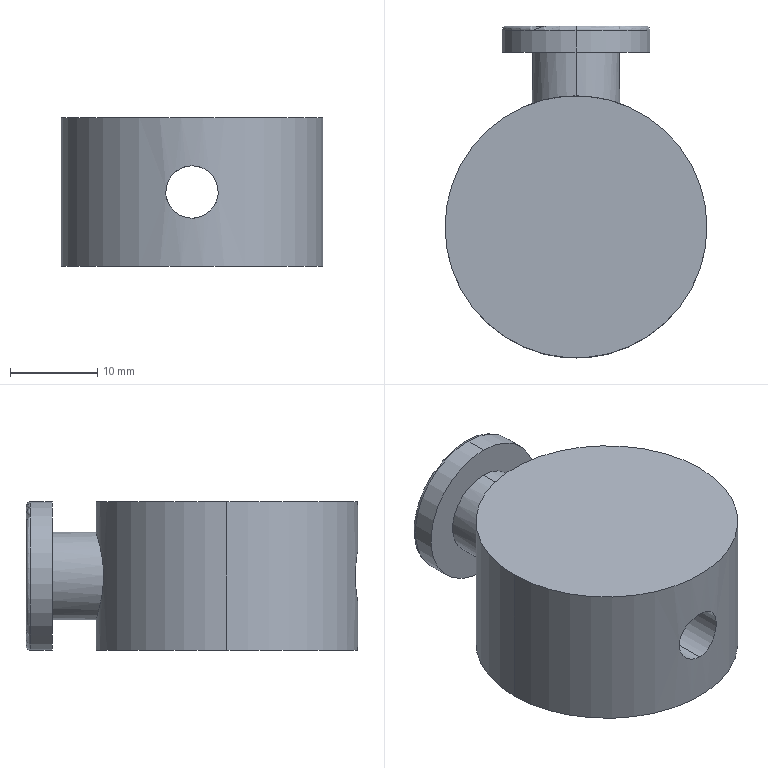Part | SolidWorks | features ICE 3, Extrusion 1, Fillet 1 | 1 solid | 14 faces | box 30 x 38 x 17 mm | volume 12032 mm3 | cylinder 8 | plane 4 | torus 2 | commonest cylinder face diameters 6 x2 10 x2 17 x2 30 x2
STEP:
#1=CARTESIAN_POINT('',(0.,22.5,-8.5));
#2=VERTEX_POINT('',#1);
#3=CARTESIAN_POINT('',(0.,22.5,8.5));
#4=VERTEX_POINT('',#3);
#5=CARTESIAN_POINT('',(0.,22.5,0.));
#6=DIRECTION('',(0.,-1.,0.));
#7=DIRECTION('',(0.,0.,1.));
#8=AXIS2_PLACEMENT_3D('',#5,#6,#7);
#9=CIRCLE('',#8,8.5);
#10=EDGE_CURVE('',#2,#4,#9,.T.);
#11=ORIENTED_EDGE('',*,*,#10,.F.);
#12=CARTESIAN_POINT('',(0.,23.,-8.));
#13=VERTEX_POINT('',#12);
#14=CARTESIAN_POINT('',(0.,22.5,-8.));
#15=DIRECTION('',(1.,0.,0.));
#16=DIRECTION('',(0.,0.,-1.));
#17=AXIS2_PLACEMENT_3D('',#14,#15,#16);
#18=CIRCLE('',#17,0.5);
#19=EDGE_CURVE('',#2,#13,#18,.T.);
#20=ORIENTED_EDGE('',*,*,#19,.T.);
#21=CARTESIAN_POINT('',(0.,23.,8.));
#22=VERTEX_POINT('',#21);
#23=CARTESIAN_POINT('',(0.,23.,0.));
#24=DIRECTION('',(0.,1.,0.));
#25=DIRECTION('',(0.,0.,1.));
#26=AXIS2_PLACEMENT_3D('',#23,#24,#25);
#27=CIRCLE('',#26,8.);
#28=EDGE_CURVE('',#22,#13,#27,.T.);
#29=ORIENTED_EDGE('',*,*,#28,.F.);
#30=CARTESIAN_POINT('',(0.,22.5,8.));
#31=DIRECTION('',(-1.,0.,0.));
#32=DIRECTION('',(0.,0.,1.));
#33=AXIS2_PLACEMENT_3D('',#30,#31,#32);
#34=CIRCLE('',#33,0.5);
#35=EDGE_CURVE('',#4,#22,#34,.T.);
#36=ORIENTED_EDGE('',*,*,#35,.F.);
#37=EDGE_LOOP('',(#11,#20,#29,#36));
#38=FACE_OUTER_BOUND('',#37,.T.);
#39=CARTESIAN_POINT('',(0.,22.5,0.));
#40=DIRECTION('',(0.,1.,0.));
#41=DIRECTION('',(0.,0.,1.));
#42=AXIS2_PLACEMENT_3D('',#39,#40,#41);
#43=TOROIDAL_SURFACE('',#42,8.,0.5);
#44=ADVANCED_FACE('',(#38),#43,.T.);
#45=ORIENTED_EDGE('',*,*,#10,.T.);
#46=CARTESIAN_POINT('',(0.,20.,8.5));
#47=VERTEX_POINT('',#46);
#48=CARTESIAN_POINT('',(0.,23.,8.5));
#49=DIRECTION('',(0.,-1.,0.));
#50=VECTOR('',#49,1000.);
#51=LINE('',#48,#50);
#52=EDGE_CURVE('',#4,#47,#51,.T.);
#53=ORIENTED_EDGE('',*,*,#52,.T.);
#54=CARTESIAN_POINT('',(0.,20.,-8.5));
#55=VERTEX_POINT('',#54);
#56=CARTESIAN_POINT('',(0.,20.,0.));
#57=DIRECTION('',(0.,1.,0.));
#58=DIRECTION('',(0.,0.,1.));
#59=AXIS2_PLACEMENT_3D('',#56,#57,#58);
#60=CIRCLE('',#59,8.5);
#61=EDGE_CURVE('',#47,#55,#60,.T.);
#62=ORIENTED_EDGE('',*,*,#61,.T.);
#63=CARTESIAN_POINT('',(0.,23.,-8.5));
#64=DIRECTION('',(0.,-1.,0.));
#65=VECTOR('',#64,1000.);
#66=LINE('',#63,#65);
#67=EDGE_CURVE('',#2,#55,#66,.T.);
#68=ORIENTED_EDGE('',*,*,#67,.F.);
#69=EDGE_LOOP('',(#45,#53,#62,#68));
#70=FACE_OUTER_BOUND('',#69,.T.);
#71=CARTESIAN_POINT('',(0.,23.,0.));
#72=DIRECTION('',(0.,-1.,0.));
#73=DIRECTION('',(0.,0.,-1.));
#74=AXIS2_PLACEMENT_3D('',#71,#72,#73);
#75=CYLINDRICAL_SURFACE('',#74,8.5);
#76=ADVANCED_FACE('',(#70),#75,.T.);
#77=CARTESIAN_POINT('',(0.,15.,5.));
#78=VERTEX_POINT('',#77);
#79=CARTESIAN_POINT('',(0.,15.,-5.));
#80=VERTEX_POINT('',#79);
#81=CARTESIAN_POINT('',(0.,15.,5.));
#82=CARTESIAN_POINT('',(0.3329,15.,5.));
#83=CARTESIAN_POINT('',(0.6598,14.989,4.967));
#84=CARTESIAN_POINT('',(1.302,14.947,4.839));
#85=CARTESIAN_POINT('',(1.621,14.915,4.741));
#86=CARTESIAN_POINT('',(2.226,14.837,4.489));
#87=CARTESIAN_POINT('',(2.512,14.791,4.335));
#88=CARTESIAN_POINT('',(3.054,14.688,3.972));
#89=CARTESIAN_POINT('',(3.308,14.633,3.763));
#90=CARTESIAN_POINT('',(3.766,14.521,3.305));
#91=CARTESIAN_POINT('',(3.972,14.466,3.055));
#92=CARTESIAN_POINT('',(4.337,14.36,2.509));
#93=CARTESIAN_POINT('',(4.491,14.313,2.222));
#94=CARTESIAN_POINT('',(4.678,14.252,1.772));
#95=CARTESIAN_POINT('',(4.734,14.234,1.618));
#96=CARTESIAN_POINT('',(4.83,14.201,1.304));
#97=CARTESIAN_POINT('',(4.871,14.187,1.142));
#98=CARTESIAN_POINT('',(4.968,14.154,0.6573));
#99=CARTESIAN_POINT('',(5.,14.142,0.3313));
#100=CARTESIAN_POINT('',(5.,14.142,-0.3263));
#101=CARTESIAN_POINT('',(4.967,14.154,-0.6604));
#102=CARTESIAN_POINT('',(4.838,14.198,-1.304));
#103=CARTESIAN_POINT('',(4.743,14.231,-1.617));
#104=CARTESIAN_POINT('',(4.49,14.313,-2.225));
#105=CARTESIAN_POINT('',(4.335,14.361,-2.513));
#106=CARTESIAN_POINT('',(3.973,14.465,-3.052));
#107=CARTESIAN_POINT('',(3.764,14.522,-3.307));
#108=CARTESIAN_POINT('',(3.304,14.634,-3.767));
#109=CARTESIAN_POINT('',(3.054,14.688,-3.972));
#110=CARTESIAN_POINT('',(2.514,14.79,-4.334));
#111=CARTESIAN_POINT('',(2.221,14.838,-4.491));
#112=CARTESIAN_POINT('',(1.619,14.915,-4.742));
#113=CARTESIAN_POINT('',(1.307,14.946,-4.837));
#114=CARTESIAN_POINT('',(0.8213,14.978,-4.935));
#115=CARTESIAN_POINT('',(0.6562,14.987,-4.959));
#116=CARTESIAN_POINT('',(0.328,14.997,-4.992));
#117=CARTESIAN_POINT('',(0.164,15.,-5.));
#118=CARTESIAN_POINT('',(0.,15.,-5.));
#119=B_SPLINE_CURVE_WITH_KNOTS('',3,(#81,#82,#83,#84,#85,#86,#87,#88,#89,#90,#91,#92,#93,#94,#95,#96,#97,#98,#99,#100,#101,#102,#103,#104,#105,#106,#107,#108,#109,#110,#111,#112,#113,#114,#115,#116,#117,#118),.UNSPECIFIED.,.F.,.F.,(4,2,2,2,2,2,2,2,2,2,2,2,2,2,2,2,2,2,4),(0.,0.0009841,0.001968,0.002952,0.003936,0.004921,0.005905,0.006397,0.006889,0.007873,0.008857,0.009841,0.01083,0.01181,0.01279,0.01378,0.01476,0.01525,0.01575),.UNSPECIFIED.);
#120=EDGE_CURVE('',#78,#80,#119,.T.);
#121=ORIENTED_EDGE('',*,*,#120,.T.);
#122=CARTESIAN_POINT('',(0.,20.,-5.));
#123=VERTEX_POINT('',#122);
#124=CARTESIAN_POINT('',(0.,-15.001,-5.));
#125=DIRECTION('',(0.,1.,0.));
#126=VECTOR('',#125,1000.);
#127=LINE('',#124,#126);
#128=EDGE_CURVE('',#80,#123,#127,.T.);
#129=ORIENTED_EDGE('',*,*,#128,.T.);
#130=CARTESIAN_POINT('',(0.,20.,5.));
#131=VERTEX_POINT('',#130);
#132=CARTESIAN_POINT('',(0.,20.,0.));
#133=DIRECTION('',(0.,1.,0.));
#134=DIRECTION('',(0.,0.,1.));
#135=AXIS2_PLACEMENT_3D('',#132,#133,#134);
#136=CIRCLE('',#135,5.);
#137=EDGE_CURVE('',#131,#123,#136,.T.);
#138=ORIENTED_EDGE('',*,*,#137,.F.);
#139=CARTESIAN_POINT('',(0.,-15.001,5.));
#140=DIRECTION('',(0.,1.,0.));
#141=VECTOR('',#140,1000.);
#142=LINE('',#139,#141);
#143=EDGE_CURVE('',#78,#131,#142,.T.);
#144=ORIENTED_EDGE('',*,*,#143,.F.);
#145=EDGE_LOOP('',(#121,#129,#138,#144));
#146=FACE_OUTER_BOUND('',#145,.T.);
#147=CARTESIAN_POINT('',(0.,-15.001,0.));
#148=DIRECTION('',(0.,1.,0.));
#149=DIRECTION('',(0.,0.,1.));
#150=AXIS2_PLACEMENT_3D('',#147,#148,#149);
#151=CYLINDRICAL_SURFACE('',#150,5.);
#152=ADVANCED_FACE('',(#146),#151,.T.);
#153=CARTESIAN_POINT('',(0.,-15.,-3.));
#154=VERTEX_POINT('',#153);
#155=CARTESIAN_POINT('',(0.,-15.,3.));
#156=VERTEX_POINT('',#155);
#157=CARTESIAN_POINT('',(0.,-15.,-3.));
#158=CARTESIAN_POINT('',(-0.196,-15.,-3.));
#159=CARTESIAN_POINT('',(-0.3912,-14.996,-2.981));
#160=CARTESIAN_POINT('',(-0.7798,-14.981,-2.904));
#161=CARTESIAN_POINT('',(-0.9683,-14.97,-2.846));
#162=CARTESIAN_POINT('',(-1.329,-14.942,-2.696));
#163=CARTESIAN_POINT('',(-1.505,-14.925,-2.603));
#164=CARTESIAN_POINT('',(-1.831,-14.889,-2.384));
#165=CARTESIAN_POINT('',(-1.982,-14.869,-2.261));
#166=CARTESIAN_POINT('',(-2.258,-14.83,-1.984));
#167=CARTESIAN_POINT('',(-2.385,-14.81,-1.83));
#168=CARTESIAN_POINT('',(-2.602,-14.773,-1.506));
#169=CARTESIAN_POINT('',(-2.694,-14.756,-1.334));
#170=CARTESIAN_POINT('',(-2.846,-14.728,-0.9697));
#171=CARTESIAN_POINT('',(-2.903,-14.716,-0.78));
#172=CARTESIAN_POINT('',(-2.98,-14.701,-0.3963));
#173=CARTESIAN_POINT('',(-3.,-14.697,-0.1996));
#174=CARTESIAN_POINT('',(-3.,-14.697,0.1966));
#175=CARTESIAN_POINT('',(-2.981,-14.701,0.3917));
#176=CARTESIAN_POINT('',(-2.904,-14.716,0.7761));
#177=CARTESIAN_POINT('',(-2.847,-14.728,0.9674));
#178=CARTESIAN_POINT('',(-2.696,-14.756,1.33));
#179=CARTESIAN_POINT('',(-2.604,-14.773,1.502));
#180=CARTESIAN_POINT('',(-2.386,-14.809,1.829));
#181=CARTESIAN_POINT('',(-2.26,-14.829,1.982));
#182=CARTESIAN_POINT('',(-1.847,-14.888,2.396));
#183=CARTESIAN_POINT('',(-1.513,-14.928,2.62));
#184=CARTESIAN_POINT('',(-0.9723,-14.97,2.845));
#185=CARTESIAN_POINT('',(-0.782,-14.981,2.903));
#186=CARTESIAN_POINT('',(-0.3948,-14.996,2.98));
#187=CARTESIAN_POINT('',(-0.1987,-15.,3.));
#188=CARTESIAN_POINT('',(0.,-15.,3.));
#189=B_SPLINE_CURVE_WITH_KNOTS('',3,(#157,#158,#159,#160,#161,#162,#163,#164,#165,#166,#167,#168,#169,#170,#171,#172,#173,#174,#175,#176,#177,#178,#179,#180,#181,#182,#183,#184,#185,#186,#187,#188),.UNSPECIFIED.,.F.,.F.,(4,2,2,2,2,2,2,2,2,2,2,2,2,2,2,4),(0.009403,0.009991,0.01058,0.01117,0.01175,0.01234,0.01293,0.01352,0.0141,0.01469,0.01528,0.01587,0.01645,0.01763,0.01822,0.0188),.UNSPECIFIED.);
#190=EDGE_CURVE('',#154,#156,#189,.T.);
#191=ORIENTED_EDGE('',*,*,#190,.F.);
#192=CARTESIAN_POINT('',(0.,23.,-3.));
#193=VERTEX_POINT('',#192);
#194=CARTESIAN_POINT('',(0.,-15.,-3.));
#195=DIRECTION('',(0.,1.,0.));
#196=VECTOR('',#195,1000.);
#197=LINE('',#194,#196);
#198=EDGE_CURVE('',#154,#193,#197,.T.);
#199=ORIENTED_EDGE('',*,*,#198,.T.);
#200=CARTESIAN_POINT('',(0.,23.,3.));
#201=VERTEX_POINT('',#200);
#202=CARTESIAN_POINT('',(0.,23.,0.));
#203=DIRECTION('',(0.,1.,0.));
#204=DIRECTION('',(0.,0.,1.));
#205=AXIS2_PLACEMENT_3D('',#202,#203,#204);
#206=CIRCLE('',#205,3.);
#207=EDGE_CURVE('',#193,#201,#206,.T.);
#208=ORIENTED_EDGE('',*,*,#207,.T.);
#209=CARTESIAN_POINT('',(0.,-15.,3.));
#210=DIRECTION('',(0.,1.,0.));
#211=VECTOR('',#210,1000.);
#212=LINE('',#209,#211);
#213=EDGE_CURVE('',#156,#201,#212,.T.);
#214=ORIENTED_EDGE('',*,*,#213,.F.);
#215=EDGE_LOOP('',(#191,#199,#208,#214));
#216=FACE_OUTER_BOUND('',#215,.T.);
#217=CARTESIAN_POINT('',(0.,-15.,0.));
#218=DIRECTION('',(0.,1.,0.));
#219=DIRECTION('',(0.,0.,1.));
#220=AXIS2_PLACEMENT_3D('',#217,#218,#219);
#221=CYLINDRICAL_SURFACE('',#220,3.);
#222=ADVANCED_FACE('',(#216),#221,.F.);
#223=ORIENTED_EDGE('',*,*,#120,.F.);
#224=CARTESIAN_POINT('',(0.,15.,-5.));
#225=CARTESIAN_POINT('',(-0.3279,15.,-5.));
#226=CARTESIAN_POINT('',(-0.6581,14.989,-4.968));
#227=CARTESIAN_POINT('',(-1.307,14.947,-4.838));
#228=CARTESIAN_POINT('',(-1.619,14.915,-4.742));
#229=CARTESIAN_POINT('',(-2.223,14.838,-4.491));
#230=CARTESIAN_POINT('',(-2.515,14.79,-4.334));
#231=CARTESIAN_POINT('',(-3.055,14.688,-3.971));
#232=CARTESIAN_POINT('',(-3.305,14.633,-3.766));
#233=CARTESIAN_POINT('',(-3.767,14.521,-3.304));
#234=CARTESIAN_POINT('',(-3.974,14.465,-3.051));
#235=CARTESIAN_POINT('',(-4.335,14.361,-2.513));
#236=CARTESIAN_POINT('',(-4.49,14.313,-2.224));
#237=CARTESIAN_POINT('',(-4.743,14.231,-1.616));
#238=CARTESIAN_POINT('',(-4.838,14.199,-1.304));
#239=CARTESIAN_POINT('',(-4.967,14.154,-0.6625));
#240=CARTESIAN_POINT('',(-5.,14.142,-0.3289));
#241=CARTESIAN_POINT('',(-5.,14.142,0.3301));
#242=CARTESIAN_POINT('',(-4.968,14.154,0.6563));
#243=CARTESIAN_POINT('',(-4.871,14.187,1.141));
#244=CARTESIAN_POINT('',(-4.83,14.201,1.302));
#245=CARTESIAN_POINT('',(-4.734,14.233,1.617));
#246=CARTESIAN_POINT('',(-4.679,14.252,1.771));
#247=CARTESIAN_POINT('',(-4.491,14.313,2.223));
#248=CARTESIAN_POINT('',(-4.336,14.361,2.512));
#249=CARTESIAN_POINT('',(-3.971,14.466,3.056));
#250=CARTESIAN_POINT('',(-3.765,14.522,3.306));
#251=CARTESIAN_POINT('',(-3.307,14.633,3.764));
#252=CARTESIAN_POINT('',(-3.052,14.689,3.974));
#253=CARTESIAN_POINT('',(-2.511,14.791,4.336));
#254=CARTESIAN_POINT('',(-2.225,14.837,4.489));
#255=CARTESIAN_POINT('',(-1.772,14.896,4.678));
#256=CARTESIAN_POINT('',(-1.616,14.914,4.735));
#257=CARTESIAN_POINT('',(-1.301,14.944,4.831));
#258=CARTESIAN_POINT('',(-1.142,14.957,4.871));
#259=CARTESIAN_POINT('',(-0.6599,14.989,4.967));
#260=CARTESIAN_POINT('',(-0.3328,15.,5.));
#261=CARTESIAN_POINT('',(0.,15.,5.));
#262=B_SPLINE_CURVE_WITH_KNOTS('',3,(#224,#225,#226,#227,#228,#229,#230,#231,#232,#233,#234,#235,#236,#237,#238,#239,#240,#241,#242,#243,#244,#245,#246,#247,#248,#249,#250,#251,#252,#253,#254,#255,#256,#257,#258,#259,#260,#261),.UNSPECIFIED.,.F.,.F.,(4,2,2,2,2,2,2,2,2,2,2,2,2,2,2,2,2,2,4),(0.01575,0.01673,0.01771,0.0187,0.01968,0.02067,0.02165,0.02263,0.02362,0.0246,0.02509,0.02558,0.02657,0.02755,0.02854,0.02952,0.03001,0.0305,0.03149),.UNSPECIFIED.);
#263=EDGE_CURVE('',#80,#78,#262,.T.);
#264=ORIENTED_EDGE('',*,*,#263,.F.);
#265=EDGE_LOOP('',(#223,#264));
#266=FACE_BOUND('',#265,.T.);
#267=CARTESIAN_POINT('',(15.,0.,8.5));
#268=VERTEX_POINT('',#267);
#269=CARTESIAN_POINT('',(-15.,0.,8.5));
#270=VERTEX_POINT('',#269);
#271=CARTESIAN_POINT('',(0.,0.,8.5));
#272=DIRECTION('',(0.,0.,1.));
#273=DIRECTION('',(1.,0.,0.));
#274=AXIS2_PLACEMENT_3D('',#271,#272,#273);
#275=CIRCLE('',#274,15.);
#276=EDGE_CURVE('',#268,#270,#275,.T.);
#277=ORIENTED_EDGE('',*,*,#276,.F.);
#278=CARTESIAN_POINT('',(15.,0.,-8.5));
#279=VERTEX_POINT('',#278);
#280=CARTESIAN_POINT('',(15.,0.,8.5));
#281=DIRECTION('',(0.,0.,-1.));
#282=VECTOR('',#281,1000.);
#283=LINE('',#280,#282);
#284=EDGE_CURVE('',#268,#279,#283,.T.);
#285=ORIENTED_EDGE('',*,*,#284,.T.);
#286=CARTESIAN_POINT('',(-15.,0.,-8.5));
#287=VERTEX_POINT('',#286);
#288=CARTESIAN_POINT('',(0.,0.,-8.5));
#289=DIRECTION('',(0.,0.,1.));
#290=DIRECTION('',(1.,0.,0.));
#291=AXIS2_PLACEMENT_3D('',#288,#289,#290);
#292=CIRCLE('',#291,15.);
#293=EDGE_CURVE('',#279,#287,#292,.T.);
#294=ORIENTED_EDGE('',*,*,#293,.T.);
#295=CARTESIAN_POINT('',(-15.,0.,8.5));
#296=DIRECTION('',(0.,0.,-1.));
#297=VECTOR('',#296,1000.);
#298=LINE('',#295,#297);
#299=EDGE_CURVE('',#270,#287,#298,.T.);
#300=ORIENTED_EDGE('',*,*,#299,.F.);
#301=EDGE_LOOP('',(#277,#285,#294,#300));
#302=FACE_OUTER_BOUND('',#301,.T.);
#303=CARTESIAN_POINT('',(0.,0.,8.5));
#304=DIRECTION('',(0.,0.,-1.));
#305=DIRECTION('',(-1.,0.,0.));
#306=AXIS2_PLACEMENT_3D('',#303,#304,#305);
#307=CYLINDRICAL_SURFACE('',#306,15.);
#308=ADVANCED_FACE('',(#266,#302),#307,.T.);
#309=ORIENTED_EDGE('',*,*,#284,.F.);
#310=CARTESIAN_POINT('',(0.,0.,8.5));
#311=DIRECTION('',(0.,0.,1.));
#312=DIRECTION('',(1.,0.,0.));
#313=AXIS2_PLACEMENT_3D('',#310,#311,#312);
#314=CIRCLE('',#313,15.);
#315=EDGE_CURVE('',#270,#268,#314,.T.);
#316=ORIENTED_EDGE('',*,*,#315,.F.);
#317=ORIENTED_EDGE('',*,*,#299,.T.);
#318=CARTESIAN_POINT('',(0.,0.,-8.5));
#319=DIRECTION('',(0.,0.,1.));
#320=DIRECTION('',(1.,0.,0.));
#321=AXIS2_PLACEMENT_3D('',#318,#319,#320);
#322=CIRCLE('',#321,15.);
#323=EDGE_CURVE('',#287,#279,#322,.T.);
#324=ORIENTED_EDGE('',*,*,#323,.T.);
#325=EDGE_LOOP('',(#309,#316,#317,#324));
#326=FACE_OUTER_BOUND('',#325,.T.);
#327=CARTESIAN_POINT('',(0.,-15.,3.));
#328=CARTESIAN_POINT('',(0.1988,-15.,3.));
#329=CARTESIAN_POINT('',(0.3941,-14.996,2.98));
#330=CARTESIAN_POINT('',(0.7782,-14.981,2.904));
#331=CARTESIAN_POINT('',(0.9691,-14.97,2.846));
#332=CARTESIAN_POINT('',(1.332,-14.942,2.695));
#333=CARTESIAN_POINT('',(1.504,-14.925,2.603));
#334=CARTESIAN_POINT('',(1.83,-14.889,2.385));
#335=CARTESIAN_POINT('',(1.984,-14.869,2.259));
#336=CARTESIAN_POINT('',(2.26,-14.829,1.983));
#337=CARTESIAN_POINT('',(2.384,-14.81,1.832));
#338=CARTESIAN_POINT('',(2.603,-14.773,1.504));
#339=CARTESIAN_POINT('',(2.696,-14.756,1.33));
#340=CARTESIAN_POINT('',(2.846,-14.728,0.9696));
#341=CARTESIAN_POINT('',(2.904,-14.716,0.7799));
#342=CARTESIAN_POINT('',(2.981,-14.701,0.3924));
#343=CARTESIAN_POINT('',(3.,-14.697,0.1974));
#344=CARTESIAN_POINT('',(3.,-14.697,-0.195));
#345=CARTESIAN_POINT('',(2.98,-14.701,-0.3944));
#346=CARTESIAN_POINT('',(2.904,-14.716,-0.7796));
#347=CARTESIAN_POINT('',(2.847,-14.728,-0.9668));
#348=CARTESIAN_POINT('',(2.696,-14.756,-1.331));
#349=CARTESIAN_POINT('',(2.602,-14.773,-1.506));
#350=CARTESIAN_POINT('',(2.385,-14.81,-1.83));
#351=CARTESIAN_POINT('',(2.261,-14.829,-1.982));
#352=CARTESIAN_POINT('',(1.982,-14.869,-2.261));
#353=CARTESIAN_POINT('',(1.831,-14.889,-2.385));
#354=CARTESIAN_POINT('',(1.506,-14.925,-2.602));
#355=CARTESIAN_POINT('',(1.331,-14.942,-2.696));
#356=CARTESIAN_POINT('',(0.9679,-14.97,-2.846));
#357=CARTESIAN_POINT('',(0.7808,-14.981,-2.903));
#358=CARTESIAN_POINT('',(0.3952,-14.996,-2.98));
#359=CARTESIAN_POINT('',(0.1961,-15.,-3.));
#360=CARTESIAN_POINT('',(0.,-15.,-3.));
#361=B_SPLINE_CURVE_WITH_KNOTS('',3,(#327,#328,#329,#330,#331,#332,#333,#334,#335,#336,#337,#338,#339,#340,#341,#342,#343,#344,#345,#346,#347,#348,#349,#350,#351,#352,#353,#354,#355,#356,#357,#358,#359,#360),.UNSPECIFIED.,.F.,.F.,(4,2,2,2,2,2,2,2,2,2,2,2,2,2,2,2,4),(0.,0.0005877,0.001175,0.001763,0.002351,0.002938,0.003526,0.004114,0.004702,0.005289,0.005877,0.006465,0.007052,0.00764,0.008228,0.008815,0.009403),.UNSPECIFIED.);
#362=EDGE_CURVE('',#156,#154,#361,.T.);
#363=ORIENTED_EDGE('',*,*,#362,.T.);
#364=ORIENTED_EDGE('',*,*,#190,.T.);
#365=EDGE_LOOP('',(#363,#364));
#366=FACE_BOUND('',#365,.T.);
#367=CARTESIAN_POINT('',(0.,0.,8.5));
#368=DIRECTION('',(0.,0.,-1.));
#369=DIRECTION('',(-1.,0.,0.));
#370=AXIS2_PLACEMENT_3D('',#367,#368,#369);
#371=CYLINDRICAL_SURFACE('',#370,15.);
#372=ADVANCED_FACE('',(#326,#366),#371,.T.);
#373=ORIENTED_EDGE('',*,*,#315,.T.);
#374=ORIENTED_EDGE('',*,*,#276,.T.);
#375=EDGE_LOOP('',(#373,#374));
#376=FACE_OUTER_BOUND('',#375,.T.);
#377=CARTESIAN_POINT('',(0.,0.,8.5));
#378=DIRECTION('',(0.,0.,1.));
#379=DIRECTION('',(1.,0.,0.));
#380=AXIS2_PLACEMENT_3D('',#377,#378,#379);
#381=PLANE('',#380);
#382=ADVANCED_FACE('',(#376),#381,.T.);
#383=ORIENTED_EDGE('',*,*,#323,.F.);
#384=ORIENTED_EDGE('',*,*,#293,.F.);
#385=EDGE_LOOP('',(#383,#384));
#386=FACE_OUTER_BOUND('',#385,.T.);
#387=CARTESIAN_POINT('',(0.,0.,-8.5));
#388=DIRECTION('',(0.,0.,1.));
#389=DIRECTION('',(1.,0.,0.));
#390=AXIS2_PLACEMENT_3D('',#387,#388,#389);
#391=PLANE('',#390);
#392=ADVANCED_FACE('',(#386),#391,.F.);
#393=ORIENTED_EDGE('',*,*,#198,.F.);
#394=ORIENTED_EDGE('',*,*,#362,.F.);
#395=ORIENTED_EDGE('',*,*,#213,.T.);
#396=CARTESIAN_POINT('',(0.,23.,0.));
#397=DIRECTION('',(0.,1.,0.));
#398=DIRECTION('',(0.,0.,1.));
#399=AXIS2_PLACEMENT_3D('',#396,#397,#398);
#400=CIRCLE('',#399,3.);
#401=EDGE_CURVE('',#201,#193,#400,.T.);
#402=ORIENTED_EDGE('',*,*,#401,.T.);
#403=EDGE_LOOP('',(#393,#394,#395,#402));
#404=FACE_OUTER_BOUND('',#403,.T.);
#405=CARTESIAN_POINT('',(0.,-15.,0.));
#406=DIRECTION('',(0.,1.,0.));
#407=DIRECTION('',(0.,0.,1.));
#408=AXIS2_PLACEMENT_3D('',#405,#406,#407);
#409=CYLINDRICAL_SURFACE('',#408,3.);
#410=ADVANCED_FACE('',(#404),#409,.F.);
#411=ORIENTED_EDGE('',*,*,#128,.F.);
#412=ORIENTED_EDGE('',*,*,#263,.T.);
#413=ORIENTED_EDGE('',*,*,#143,.T.);
#414=CARTESIAN_POINT('',(0.,20.,0.));
#415=DIRECTION('',(0.,1.,0.));
#416=DIRECTION('',(0.,0.,1.));
#417=AXIS2_PLACEMENT_3D('',#414,#415,#416);
#418=CIRCLE('',#417,5.);
#419=EDGE_CURVE('',#123,#131,#418,.T.);
#420=ORIENTED_EDGE('',*,*,#419,.F.);
#421=EDGE_LOOP('',(#411,#412,#413,#420));
#422=FACE_OUTER_BOUND('',#421,.T.);
#423=CARTESIAN_POINT('',(0.,-15.001,0.));
#424=DIRECTION('',(0.,1.,0.));
#425=DIRECTION('',(0.,0.,1.));
#426=AXIS2_PLACEMENT_3D('',#423,#424,#425);
#427=CYLINDRICAL_SURFACE('',#426,5.);
#428=ADVANCED_FACE('',(#422),#427,.T.);
#429=ORIENTED_EDGE('',*,*,#28,.T.);
#430=CARTESIAN_POINT('',(0.,23.,0.));
#431=DIRECTION('',(0.,1.,0.));
#432=DIRECTION('',(0.,0.,1.));
#433=AXIS2_PLACEMENT_3D('',#430,#431,#432);
#434=CIRCLE('',#433,8.);
#435=EDGE_CURVE('',#13,#22,#434,.T.);
#436=ORIENTED_EDGE('',*,*,#435,.T.);
#437=EDGE_LOOP('',(#429,#436));
#438=FACE_OUTER_BOUND('',#437,.T.);
#439=ORIENTED_EDGE('',*,*,#401,.F.);
#440=ORIENTED_EDGE('',*,*,#207,.F.);
#441=EDGE_LOOP('',(#439,#440));
#442=FACE_BOUND('',#441,.T.);
#443=CARTESIAN_POINT('',(0.,23.,0.));
#444=DIRECTION('',(0.,1.,0.));
#445=DIRECTION('',(0.,0.,1.));
#446=AXIS2_PLACEMENT_3D('',#443,#444,#445);
#447=PLANE('',#446);
#448=ADVANCED_FACE('',(#438,#442),#447,.T.);
#449=ORIENTED_EDGE('',*,*,#137,.T.);
#450=ORIENTED_EDGE('',*,*,#419,.T.);
#451=EDGE_LOOP('',(#449,#450));
#452=FACE_BOUND('',#451,.T.);
#453=CARTESIAN_POINT('',(0.,20.,0.));
#454=DIRECTION('',(0.,1.,0.));
#455=DIRECTION('',(0.,0.,1.));
#456=AXIS2_PLACEMENT_3D('',#453,#454,#455);
#457=CIRCLE('',#456,8.5);
#458=EDGE_CURVE('',#55,#47,#457,.T.);
#459=ORIENTED_EDGE('',*,*,#458,.F.);
#460=ORIENTED_EDGE('',*,*,#61,.F.);
#461=EDGE_LOOP('',(#459,#460));
#462=FACE_OUTER_BOUND('',#461,.T.);
#463=CARTESIAN_POINT('',(0.,20.,0.));
#464=DIRECTION('',(0.,1.,0.));
#465=DIRECTION('',(0.,0.,1.));
#466=AXIS2_PLACEMENT_3D('',#463,#464,#465);
#467=PLANE('',#466);
#468=ADVANCED_FACE('',(#452,#462),#467,.F.);
#469=ORIENTED_EDGE('',*,*,#52,.F.);
#470=CARTESIAN_POINT('',(0.,22.5,0.));
#471=DIRECTION('',(0.,-1.,0.));
#472=DIRECTION('',(0.,0.,1.));
#473=AXIS2_PLACEMENT_3D('',#470,#471,#472);
#474=CIRCLE('',#473,8.5);
#475=EDGE_CURVE('',#4,#2,#474,.T.);
#476=ORIENTED_EDGE('',*,*,#475,.T.);
#477=ORIENTED_EDGE('',*,*,#67,.T.);
#478=ORIENTED_EDGE('',*,*,#458,.T.);
#479=EDGE_LOOP('',(#469,#476,#477,#478));
#480=FACE_OUTER_BOUND('',#479,.T.);
#481=CARTESIAN_POINT('',(0.,23.,0.));
#482=DIRECTION('',(0.,-1.,0.));
#483=DIRECTION('',(0.,0.,-1.));
#484=AXIS2_PLACEMENT_3D('',#481,#482,#483);
#485=CYLINDRICAL_SURFACE('',#484,8.5);
#486=ADVANCED_FACE('',(#480),#485,.T.);
#487=ORIENTED_EDGE('',*,*,#19,.F.);
#488=ORIENTED_EDGE('',*,*,#475,.F.);
#489=ORIENTED_EDGE('',*,*,#35,.T.);
#490=ORIENTED_EDGE('',*,*,#435,.F.);
#491=EDGE_LOOP('',(#487,#488,#489,#490));
#492=FACE_OUTER_BOUND('',#491,.T.);
#493=CARTESIAN_POINT('',(0.,22.5,0.));
#494=DIRECTION('',(0.,1.,0.));
#495=DIRECTION('',(0.,0.,1.));
#496=AXIS2_PLACEMENT_3D('',#493,#494,#495);
#497=TOROIDAL_SURFACE('',#496,8.,0.5);
#498=ADVANCED_FACE('',(#492),#497,.T.);
#499=CLOSED_SHELL('',(#44,#76,#152,#222,#308,#372,#382,#392,#410,#428,#448,#468,#486,#498));
#500=MANIFOLD_SOLID_BREP('',#499);
#501=CARTESIAN_POINT('',(0.,0.,0.));
#502=DIRECTION('',(0.,0.,1.));
#503=DIRECTION('',(1.,0.,0.));
#504=AXIS2_PLACEMENT_3D('',#501,#502,#503);
#505=(LENGTH_UNIT()NAMED_UNIT(*)SI_UNIT(.MILLI.,.METRE.));
#506=UNCERTAINTY_MEASURE_WITH_UNIT(LENGTH_MEASURE(0.00001),#505,'','');
#507=(NAMED_UNIT(*)PLANE_ANGLE_UNIT()SI_UNIT($,.RADIAN.));
#508=(NAMED_UNIT(*)SI_UNIT($,.STERADIAN.)SOLID_ANGLE_UNIT());
#509=(GEOMETRIC_REPRESENTATION_CONTEXT(3)GLOBAL_UNCERTAINTY_ASSIGNED_CONTEXT((#506))GLOBAL_UNIT_ASSIGNED_CONTEXT((#505,#507,#508))REPRESENTATION_CONTEXT('',''));
#510=ADVANCED_BREP_SHAPE_REPRESENTATION('',(#500,#504),#509);